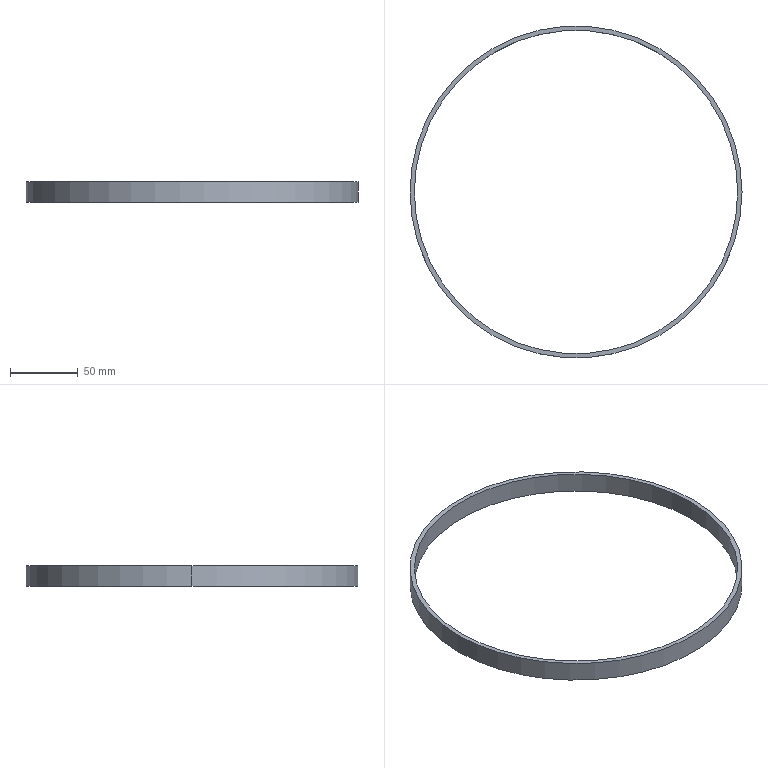Part | SolidWorks | features Extrusion 1 | 1 solid | 6 faces | box 244.5 x 244.5 x 15 mm | volume 36387 mm3 | cylinder 4 | plane 2 | commonest cylinder face diameters 238.1 x2 244.5 x2
STEP:
#1=CARTESIAN_POINT('',(-119.05,0.,15.));
#2=VERTEX_POINT('',#1);
#3=CARTESIAN_POINT('',(119.05,0.,15.));
#4=VERTEX_POINT('',#3);
#5=CARTESIAN_POINT('',(0.,0.,15.));
#6=DIRECTION('',(0.,0.,1.));
#7=DIRECTION('',(1.,0.,0.));
#8=AXIS2_PLACEMENT_3D('',#5,#6,#7);
#9=CIRCLE('',#8,119.05);
#10=EDGE_CURVE('',#2,#4,#9,.T.);
#11=ORIENTED_EDGE('',*,*,#10,.T.);
#12=CARTESIAN_POINT('',(119.05,0.,0.));
#13=VERTEX_POINT('',#12);
#14=CARTESIAN_POINT('',(119.05,0.,15.));
#15=DIRECTION('',(0.,0.,-1.));
#16=VECTOR('',#15,1000.);
#17=LINE('',#14,#16);
#18=EDGE_CURVE('',#4,#13,#17,.T.);
#19=ORIENTED_EDGE('',*,*,#18,.T.);
#20=CARTESIAN_POINT('',(-119.05,0.,0.));
#21=VERTEX_POINT('',#20);
#22=CARTESIAN_POINT('',(0.,0.,0.));
#23=DIRECTION('',(0.,0.,1.));
#24=DIRECTION('',(1.,0.,0.));
#25=AXIS2_PLACEMENT_3D('',#22,#23,#24);
#26=CIRCLE('',#25,119.05);
#27=EDGE_CURVE('',#21,#13,#26,.T.);
#28=ORIENTED_EDGE('',*,*,#27,.F.);
#29=CARTESIAN_POINT('',(-119.05,0.,15.));
#30=DIRECTION('',(0.,0.,-1.));
#31=VECTOR('',#30,1000.);
#32=LINE('',#29,#31);
#33=EDGE_CURVE('',#2,#21,#32,.T.);
#34=ORIENTED_EDGE('',*,*,#33,.F.);
#35=EDGE_LOOP('',(#11,#19,#28,#34));
#36=FACE_OUTER_BOUND('',#35,.T.);
#37=CARTESIAN_POINT('',(0.,0.,15.));
#38=DIRECTION('',(0.,0.,-1.));
#39=DIRECTION('',(-1.,0.,0.));
#40=AXIS2_PLACEMENT_3D('',#37,#38,#39);
#41=CYLINDRICAL_SURFACE('',#40,119.05);
#42=ADVANCED_FACE('',(#36),#41,.F.);
#43=CARTESIAN_POINT('',(122.25,0.,15.));
#44=VERTEX_POINT('',#43);
#45=CARTESIAN_POINT('',(-122.25,0.,15.));
#46=VERTEX_POINT('',#45);
#47=CARTESIAN_POINT('',(0.,0.,15.));
#48=DIRECTION('',(0.,0.,1.));
#49=DIRECTION('',(1.,0.,0.));
#50=AXIS2_PLACEMENT_3D('',#47,#48,#49);
#51=CIRCLE('',#50,122.25);
#52=EDGE_CURVE('',#44,#46,#51,.T.);
#53=ORIENTED_EDGE('',*,*,#52,.F.);
#54=CARTESIAN_POINT('',(122.25,0.,0.));
#55=VERTEX_POINT('',#54);
#56=CARTESIAN_POINT('',(122.25,0.,15.));
#57=DIRECTION('',(0.,0.,-1.));
#58=VECTOR('',#57,1000.);
#59=LINE('',#56,#58);
#60=EDGE_CURVE('',#44,#55,#59,.T.);
#61=ORIENTED_EDGE('',*,*,#60,.T.);
#62=CARTESIAN_POINT('',(-122.25,0.,0.));
#63=VERTEX_POINT('',#62);
#64=CARTESIAN_POINT('',(0.,0.,0.));
#65=DIRECTION('',(0.,0.,1.));
#66=DIRECTION('',(1.,0.,0.));
#67=AXIS2_PLACEMENT_3D('',#64,#65,#66);
#68=CIRCLE('',#67,122.25);
#69=EDGE_CURVE('',#55,#63,#68,.T.);
#70=ORIENTED_EDGE('',*,*,#69,.T.);
#71=CARTESIAN_POINT('',(-122.25,0.,15.));
#72=DIRECTION('',(0.,0.,-1.));
#73=VECTOR('',#72,1000.);
#74=LINE('',#71,#73);
#75=EDGE_CURVE('',#46,#63,#74,.T.);
#76=ORIENTED_EDGE('',*,*,#75,.F.);
#77=EDGE_LOOP('',(#53,#61,#70,#76));
#78=FACE_OUTER_BOUND('',#77,.T.);
#79=CARTESIAN_POINT('',(0.,0.,15.));
#80=DIRECTION('',(0.,0.,-1.));
#81=DIRECTION('',(-1.,0.,0.));
#82=AXIS2_PLACEMENT_3D('',#79,#80,#81);
#83=CYLINDRICAL_SURFACE('',#82,122.25);
#84=ADVANCED_FACE('',(#78),#83,.T.);
#85=CARTESIAN_POINT('',(0.,0.,15.));
#86=DIRECTION('',(0.,0.,1.));
#87=DIRECTION('',(1.,0.,0.));
#88=AXIS2_PLACEMENT_3D('',#85,#86,#87);
#89=CIRCLE('',#88,122.25);
#90=EDGE_CURVE('',#46,#44,#89,.T.);
#91=ORIENTED_EDGE('',*,*,#90,.T.);
#92=ORIENTED_EDGE('',*,*,#52,.T.);
#93=EDGE_LOOP('',(#91,#92));
#94=FACE_OUTER_BOUND('',#93,.T.);
#95=ORIENTED_EDGE('',*,*,#10,.F.);
#96=CARTESIAN_POINT('',(0.,0.,15.));
#97=DIRECTION('',(0.,0.,1.));
#98=DIRECTION('',(1.,0.,0.));
#99=AXIS2_PLACEMENT_3D('',#96,#97,#98);
#100=CIRCLE('',#99,119.05);
#101=EDGE_CURVE('',#4,#2,#100,.T.);
#102=ORIENTED_EDGE('',*,*,#101,.F.);
#103=EDGE_LOOP('',(#95,#102));
#104=FACE_BOUND('',#103,.T.);
#105=CARTESIAN_POINT('',(0.,0.,15.));
#106=DIRECTION('',(0.,0.,1.));
#107=DIRECTION('',(1.,0.,0.));
#108=AXIS2_PLACEMENT_3D('',#105,#106,#107);
#109=PLANE('',#108);
#110=ADVANCED_FACE('',(#94,#104),#109,.T.);
#111=CARTESIAN_POINT('',(0.,0.,0.));
#112=DIRECTION('',(0.,0.,1.));
#113=DIRECTION('',(1.,0.,0.));
#114=AXIS2_PLACEMENT_3D('',#111,#112,#113);
#115=CIRCLE('',#114,122.25);
#116=EDGE_CURVE('',#63,#55,#115,.T.);
#117=ORIENTED_EDGE('',*,*,#116,.F.);
#118=ORIENTED_EDGE('',*,*,#69,.F.);
#119=EDGE_LOOP('',(#117,#118));
#120=FACE_OUTER_BOUND('',#119,.T.);
#121=ORIENTED_EDGE('',*,*,#27,.T.);
#122=CARTESIAN_POINT('',(0.,0.,0.));
#123=DIRECTION('',(0.,0.,1.));
#124=DIRECTION('',(1.,0.,0.));
#125=AXIS2_PLACEMENT_3D('',#122,#123,#124);
#126=CIRCLE('',#125,119.05);
#127=EDGE_CURVE('',#13,#21,#126,.T.);
#128=ORIENTED_EDGE('',*,*,#127,.T.);
#129=EDGE_LOOP('',(#121,#128));
#130=FACE_BOUND('',#129,.T.);
#131=CARTESIAN_POINT('',(0.,0.,0.));
#132=DIRECTION('',(0.,0.,1.));
#133=DIRECTION('',(1.,0.,0.));
#134=AXIS2_PLACEMENT_3D('',#131,#132,#133);
#135=PLANE('',#134);
#136=ADVANCED_FACE('',(#120,#130),#135,.F.);
#137=ORIENTED_EDGE('',*,*,#60,.F.);
#138=ORIENTED_EDGE('',*,*,#90,.F.);
#139=ORIENTED_EDGE('',*,*,#75,.T.);
#140=ORIENTED_EDGE('',*,*,#116,.T.);
#141=EDGE_LOOP('',(#137,#138,#139,#140));
#142=FACE_OUTER_BOUND('',#141,.T.);
#143=CARTESIAN_POINT('',(0.,0.,15.));
#144=DIRECTION('',(0.,0.,-1.));
#145=DIRECTION('',(-1.,0.,0.));
#146=AXIS2_PLACEMENT_3D('',#143,#144,#145);
#147=CYLINDRICAL_SURFACE('',#146,122.25);
#148=ADVANCED_FACE('',(#142),#147,.T.);
#149=ORIENTED_EDGE('',*,*,#18,.F.);
#150=ORIENTED_EDGE('',*,*,#101,.T.);
#151=ORIENTED_EDGE('',*,*,#33,.T.);
#152=ORIENTED_EDGE('',*,*,#127,.F.);
#153=EDGE_LOOP('',(#149,#150,#151,#152));
#154=FACE_OUTER_BOUND('',#153,.T.);
#155=CARTESIAN_POINT('',(0.,0.,15.));
#156=DIRECTION('',(0.,0.,-1.));
#157=DIRECTION('',(-1.,0.,0.));
#158=AXIS2_PLACEMENT_3D('',#155,#156,#157);
#159=CYLINDRICAL_SURFACE('',#158,119.05);
#160=ADVANCED_FACE('',(#154),#159,.F.);
#161=CLOSED_SHELL('',(#42,#84,#110,#136,#148,#160));
#162=MANIFOLD_SOLID_BREP('',#161);
#163=CARTESIAN_POINT('',(0.,0.,0.));
#164=DIRECTION('',(0.,0.,1.));
#165=DIRECTION('',(1.,0.,0.));
#166=AXIS2_PLACEMENT_3D('',#163,#164,#165);
#167=(LENGTH_UNIT()NAMED_UNIT(*)SI_UNIT(.MILLI.,.METRE.));
#168=UNCERTAINTY_MEASURE_WITH_UNIT(LENGTH_MEASURE(0.00001),#167,'','');
#169=(NAMED_UNIT(*)PLANE_ANGLE_UNIT()SI_UNIT($,.RADIAN.));
#170=(NAMED_UNIT(*)SI_UNIT($,.STERADIAN.)SOLID_ANGLE_UNIT());
#171=(GEOMETRIC_REPRESENTATION_CONTEXT(3)GLOBAL_UNCERTAINTY_ASSIGNED_CONTEXT((#168))GLOBAL_UNIT_ASSIGNED_CONTEXT((#167,#169,#170))REPRESENTATION_CONTEXT('',''));
#172=ADVANCED_BREP_SHAPE_REPRESENTATION('',(#162,#166),#171);